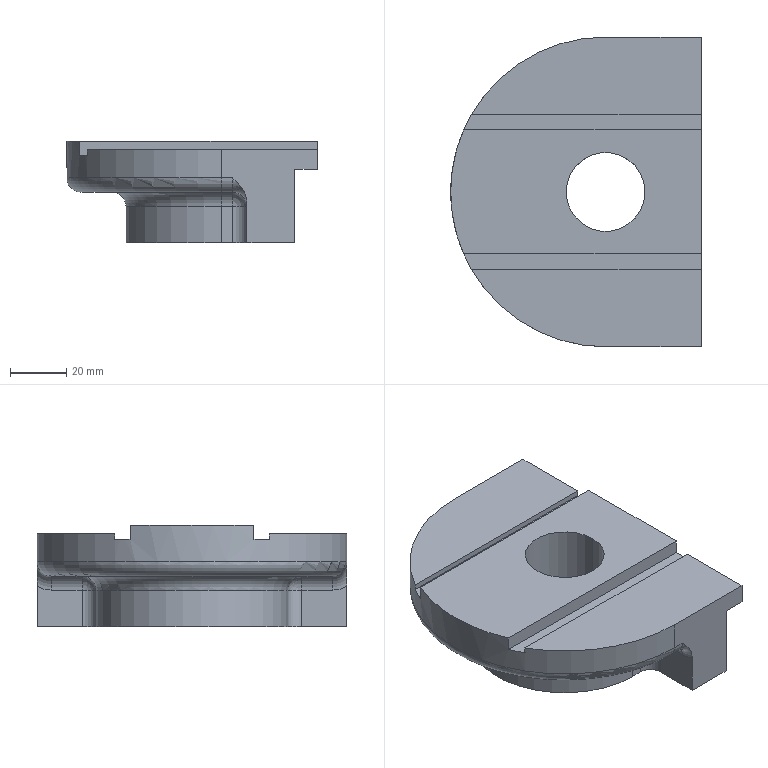Part | SolidWorks | features ICE 6, Fillet 3, Extrusion 1, MirrorPattern 1, RevCut 1 | 1 solid | 49 faces | box 89 x 110 x 36 mm | volume 178955 mm3 | plane 21 | cylinder 18 | cone 4 | torus 4 | sphere 2 | commonest cylinder face diameters 10 x8 5.5 x4 28 x2 36 x2 68 x1 110 x1
STEP:
#1=CARTESIAN_POINT('',(11.,-38.,-25.75));
#2=VERTEX_POINT('',#1);
#3=CARTESIAN_POINT('',(11.,-38.,-20.25));
#4=VERTEX_POINT('',#3);
#5=CARTESIAN_POINT('',(11.,-38.,-23.));
#6=DIRECTION('',(-1.,0.,0.));
#7=DIRECTION('',(0.,0.,-1.));
#8=AXIS2_PLACEMENT_3D('',#5,#6,#7);
#9=CIRCLE('',#8,2.75);
#10=EDGE_CURVE('',#2,#4,#9,.T.);
#11=ORIENTED_EDGE('',*,*,#10,.T.);
#12=CARTESIAN_POINT('',(26.,-38.,-20.25));
#13=VERTEX_POINT('',#12);
#14=CARTESIAN_POINT('',(29.177,-38.,-20.25));
#15=DIRECTION('',(1.,0.,0.));
#16=VECTOR('',#15,1000.);
#17=LINE('',#14,#16);
#18=EDGE_CURVE('',#4,#13,#17,.T.);
#19=ORIENTED_EDGE('',*,*,#18,.T.);
#20=CARTESIAN_POINT('',(26.,-38.,-25.75));
#21=VERTEX_POINT('',#20);
#22=CARTESIAN_POINT('',(26.,-38.,-23.));
#23=DIRECTION('',(-1.,0.,0.));
#24=DIRECTION('',(0.,0.,-1.));
#25=AXIS2_PLACEMENT_3D('',#22,#23,#24);
#26=CIRCLE('',#25,2.75);
#27=EDGE_CURVE('',#21,#13,#26,.T.);
#28=ORIENTED_EDGE('',*,*,#27,.F.);
#29=CARTESIAN_POINT('',(29.177,-38.,-25.75));
#30=DIRECTION('',(1.,0.,0.));
#31=VECTOR('',#30,1000.);
#32=LINE('',#29,#31);
#33=EDGE_CURVE('',#2,#21,#32,.T.);
#34=ORIENTED_EDGE('',*,*,#33,.F.);
#35=EDGE_LOOP('',(#11,#19,#28,#34));
#36=FACE_OUTER_BOUND('',#35,.T.);
#37=CARTESIAN_POINT('',(29.177,-38.,-23.));
#38=DIRECTION('',(1.,0.,0.));
#39=DIRECTION('',(0.,0.,-1.));
#40=AXIS2_PLACEMENT_3D('',#37,#38,#39);
#41=CYLINDRICAL_SURFACE('',#40,2.75);
#42=ADVANCED_FACE('',(#36),#41,.F.);
#43=CARTESIAN_POINT('',(9.412,-38.,-23.));
#44=VERTEX_POINT('',#43);
#45=CARTESIAN_POINT('',(9.412,-38.,-23.));
#46=DIRECTION('',(0.5,0.,-0.866));
#47=VECTOR('',#46,1000.);
#48=LINE('',#45,#47);
#49=EDGE_CURVE('',#44,#2,#48,.T.);
#50=ORIENTED_EDGE('',*,*,#49,.F.);
#51=CARTESIAN_POINT('',(9.412,-38.,-23.));
#52=DIRECTION('',(0.5,0.,0.866));
#53=VECTOR('',#52,1000.);
#54=LINE('',#51,#53);
#55=EDGE_CURVE('',#44,#4,#54,.T.);
#56=ORIENTED_EDGE('',*,*,#55,.T.);
#57=ORIENTED_EDGE('',*,*,#10,.F.);
#58=EDGE_LOOP('',(#50,#56,#57));
#59=FACE_OUTER_BOUND('',#58,.T.);
#60=CARTESIAN_POINT('',(1009.412,-38.,-23.));
#61=DIRECTION('',(1.,0.,0.));
#62=DIRECTION('',(0.,0.,-1.));
#63=AXIS2_PLACEMENT_3D('',#60,#61,#62);
#64=CONICAL_SURFACE('',#63,1732.051,1.047);
#65=ADVANCED_FACE('',(#59),#64,.F.);
#66=CARTESIAN_POINT('',(11.,38.,-20.25));
#67=VERTEX_POINT('',#66);
#68=CARTESIAN_POINT('',(11.,38.,-25.75));
#69=VERTEX_POINT('',#68);
#70=CARTESIAN_POINT('',(11.,38.,-23.));
#71=DIRECTION('',(1.,0.,0.));
#72=DIRECTION('',(0.,0.,-1.));
#73=AXIS2_PLACEMENT_3D('',#70,#71,#72);
#74=CIRCLE('',#73,2.75);
#75=EDGE_CURVE('',#67,#69,#74,.T.);
#76=ORIENTED_EDGE('',*,*,#75,.F.);
#77=CARTESIAN_POINT('',(26.,38.,-20.25));
#78=VERTEX_POINT('',#77);
#79=CARTESIAN_POINT('',(29.177,38.,-20.25));
#80=DIRECTION('',(1.,0.,0.));
#81=VECTOR('',#80,1000.);
#82=LINE('',#79,#81);
#83=EDGE_CURVE('',#67,#78,#82,.T.);
#84=ORIENTED_EDGE('',*,*,#83,.T.);
#85=CARTESIAN_POINT('',(26.,38.,-25.75));
#86=VERTEX_POINT('',#85);
#87=CARTESIAN_POINT('',(26.,38.,-23.));
#88=DIRECTION('',(1.,0.,0.));
#89=DIRECTION('',(0.,0.,-1.));
#90=AXIS2_PLACEMENT_3D('',#87,#88,#89);
#91=CIRCLE('',#90,2.75);
#92=EDGE_CURVE('',#78,#86,#91,.T.);
#93=ORIENTED_EDGE('',*,*,#92,.T.);
#94=CARTESIAN_POINT('',(29.177,38.,-25.75));
#95=DIRECTION('',(1.,0.,0.));
#96=VECTOR('',#95,1000.);
#97=LINE('',#94,#96);
#98=EDGE_CURVE('',#69,#86,#97,.T.);
#99=ORIENTED_EDGE('',*,*,#98,.F.);
#100=EDGE_LOOP('',(#76,#84,#93,#99));
#101=FACE_OUTER_BOUND('',#100,.T.);
#102=CARTESIAN_POINT('',(29.177,38.,-23.));
#103=DIRECTION('',(1.,0.,0.));
#104=DIRECTION('',(0.,0.,-1.));
#105=AXIS2_PLACEMENT_3D('',#102,#103,#104);
#106=CYLINDRICAL_SURFACE('',#105,2.75);
#107=ADVANCED_FACE('',(#101),#106,.F.);
#108=CARTESIAN_POINT('',(9.412,38.,-23.));
#109=VERTEX_POINT('',#108);
#110=CARTESIAN_POINT('',(9.412,38.,-23.));
#111=DIRECTION('',(0.5,0.,-0.866));
#112=VECTOR('',#111,1000.);
#113=LINE('',#110,#112);
#114=EDGE_CURVE('',#109,#69,#113,.T.);
#115=ORIENTED_EDGE('',*,*,#114,.F.);
#116=CARTESIAN_POINT('',(9.412,38.,-23.));
#117=DIRECTION('',(0.5,0.,0.866));
#118=VECTOR('',#117,1000.);
#119=LINE('',#116,#118);
#120=EDGE_CURVE('',#109,#67,#119,.T.);
#121=ORIENTED_EDGE('',*,*,#120,.T.);
#122=ORIENTED_EDGE('',*,*,#75,.T.);
#123=EDGE_LOOP('',(#115,#121,#122));
#124=FACE_OUTER_BOUND('',#123,.T.);
#125=CARTESIAN_POINT('',(1009.412,38.,-23.));
#126=DIRECTION('',(1.,0.,0.));
#127=DIRECTION('',(0.,0.,-1.));
#128=AXIS2_PLACEMENT_3D('',#125,#126,#127);
#129=CONICAL_SURFACE('',#128,1732.051,1.047);
#130=ADVANCED_FACE('',(#124),#129,.F.);
#131=CARTESIAN_POINT('',(18.,0.,-22.));
#132=VERTEX_POINT('',#131);
#133=CARTESIAN_POINT('',(-18.,0.,-22.));
#134=VERTEX_POINT('',#133);
#135=CARTESIAN_POINT('',(0.,0.,-22.));
#136=DIRECTION('',(0.,0.,-1.));
#137=DIRECTION('',(-1.,0.,0.));
#138=AXIS2_PLACEMENT_3D('',#135,#136,#137);
#139=CIRCLE('',#138,18.);
#140=EDGE_CURVE('',#132,#134,#139,.T.);
#141=ORIENTED_EDGE('',*,*,#140,.F.);
#142=CARTESIAN_POINT('',(18.,0.,-36.));
#143=VERTEX_POINT('',#142);
#144=CARTESIAN_POINT('',(18.,0.,-22.));
#145=DIRECTION('',(0.,0.,-1.));
#146=VECTOR('',#145,1000.);
#147=LINE('',#144,#146);
#148=EDGE_CURVE('',#132,#143,#147,.T.);
#149=ORIENTED_EDGE('',*,*,#148,.T.);
#150=CARTESIAN_POINT('',(-18.,0.,-36.));
#151=VERTEX_POINT('',#150);
#152=CARTESIAN_POINT('',(0.,0.,-36.));
#153=DIRECTION('',(0.,0.,-1.));
#154=DIRECTION('',(-1.,0.,0.));
#155=AXIS2_PLACEMENT_3D('',#152,#153,#154);
#156=CIRCLE('',#155,18.);
#157=EDGE_CURVE('',#143,#151,#156,.T.);
#158=ORIENTED_EDGE('',*,*,#157,.T.);
#159=CARTESIAN_POINT('',(-18.,0.,-22.));
#160=DIRECTION('',(0.,0.,-1.));
#161=VECTOR('',#160,1000.);
#162=LINE('',#159,#161);
#163=EDGE_CURVE('',#134,#151,#162,.T.);
#164=ORIENTED_EDGE('',*,*,#163,.F.);
#165=EDGE_LOOP('',(#141,#149,#158,#164));
#166=FACE_OUTER_BOUND('',#165,.T.);
#167=CARTESIAN_POINT('',(0.,0.,-22.));
#168=DIRECTION('',(0.,0.,-1.));
#169=DIRECTION('',(-1.,0.,0.));
#170=AXIS2_PLACEMENT_3D('',#167,#168,#169);
#171=CYLINDRICAL_SURFACE('',#170,18.);
#172=ADVANCED_FACE('',(#166),#171,.F.);
#173=CARTESIAN_POINT('',(-14.,0.,0.));
#174=VERTEX_POINT('',#173);
#175=CARTESIAN_POINT('',(14.,0.,0.));
#176=VERTEX_POINT('',#175);
#177=CARTESIAN_POINT('',(0.,0.,0.));
#178=DIRECTION('',(0.,0.,1.));
#179=DIRECTION('',(1.,0.,0.));
#180=AXIS2_PLACEMENT_3D('',#177,#178,#179);
#181=CIRCLE('',#180,14.);
#182=EDGE_CURVE('',#174,#176,#181,.T.);
#183=ORIENTED_EDGE('',*,*,#182,.T.);
#184=CARTESIAN_POINT('',(14.,0.,-22.));
#185=VERTEX_POINT('',#184);
#186=CARTESIAN_POINT('',(14.,0.,1.));
#187=DIRECTION('',(0.,0.,-1.));
#188=VECTOR('',#187,1000.);
#189=LINE('',#186,#188);
#190=EDGE_CURVE('',#176,#185,#189,.T.);
#191=ORIENTED_EDGE('',*,*,#190,.T.);
#192=CARTESIAN_POINT('',(-14.,0.,-22.));
#193=VERTEX_POINT('',#192);
#194=CARTESIAN_POINT('',(0.,0.,-22.));
#195=DIRECTION('',(0.,0.,1.));
#196=DIRECTION('',(-1.,0.,0.));
#197=AXIS2_PLACEMENT_3D('',#194,#195,#196);
#198=CIRCLE('',#197,14.);
#199=EDGE_CURVE('',#193,#185,#198,.T.);
#200=ORIENTED_EDGE('',*,*,#199,.F.);
#201=CARTESIAN_POINT('',(-14.,0.,1.));
#202=DIRECTION('',(0.,0.,-1.));
#203=VECTOR('',#202,1000.);
#204=LINE('',#201,#203);
#205=EDGE_CURVE('',#174,#193,#204,.T.);
#206=ORIENTED_EDGE('',*,*,#205,.F.);
#207=EDGE_LOOP('',(#183,#191,#200,#206));
#208=FACE_OUTER_BOUND('',#207,.T.);
#209=CARTESIAN_POINT('',(0.,0.,1.));
#210=DIRECTION('',(0.,0.,-1.));
#211=DIRECTION('',(-1.,0.,0.));
#212=AXIS2_PLACEMENT_3D('',#209,#210,#211);
#213=CYLINDRICAL_SURFACE('',#212,14.);
#214=ADVANCED_FACE('',(#208),#213,.F.);
#215=CARTESIAN_POINT('',(34.,-55.,-10.));
#216=VERTEX_POINT('',#215);
#217=CARTESIAN_POINT('',(34.,-55.,-3.));
#218=VERTEX_POINT('',#217);
#219=CARTESIAN_POINT('',(34.,-55.,-18.));
#220=DIRECTION('',(0.,0.,1.));
#221=VECTOR('',#220,1000.);
#222=LINE('',#219,#221);
#223=EDGE_CURVE('',#216,#218,#222,.T.);
#224=ORIENTED_EDGE('',*,*,#223,.F.);
#225=CARTESIAN_POINT('',(34.,55.,-10.));
#226=VERTEX_POINT('',#225);
#227=CARTESIAN_POINT('',(34.,55.,-10.));
#228=DIRECTION('',(0.,-1.,0.));
#229=VECTOR('',#228,1000.);
#230=LINE('',#227,#229);
#231=EDGE_CURVE('',#226,#216,#230,.T.);
#232=ORIENTED_EDGE('',*,*,#231,.F.);
#233=CARTESIAN_POINT('',(34.,55.,-3.));
#234=VERTEX_POINT('',#233);
#235=CARTESIAN_POINT('',(34.,55.,-18.));
#236=DIRECTION('',(0.,0.,1.));
#237=VECTOR('',#236,1000.);
#238=LINE('',#235,#237);
#239=EDGE_CURVE('',#226,#234,#238,.T.);
#240=ORIENTED_EDGE('',*,*,#239,.T.);
#241=CARTESIAN_POINT('',(34.,27.5,-3.));
#242=VERTEX_POINT('',#241);
#243=CARTESIAN_POINT('',(34.,55.,-3.));
#244=DIRECTION('',(0.,1.,0.));
#245=VECTOR('',#244,1000.);
#246=LINE('',#243,#245);
#247=EDGE_CURVE('',#242,#234,#246,.T.);
#248=ORIENTED_EDGE('',*,*,#247,.F.);
#249=CARTESIAN_POINT('',(34.,27.5,-5.));
#250=VERTEX_POINT('',#249);
#251=CARTESIAN_POINT('',(34.,27.5,0.));
#252=DIRECTION('',(0.,0.,1.));
#253=VECTOR('',#252,1000.);
#254=LINE('',#251,#253);
#255=EDGE_CURVE('',#250,#242,#254,.T.);
#256=ORIENTED_EDGE('',*,*,#255,.F.);
#257=CARTESIAN_POINT('',(34.,22.,-5.));
#258=VERTEX_POINT('',#257);
#259=CARTESIAN_POINT('',(34.,22.,-5.));
#260=DIRECTION('',(0.,1.,0.));
#261=VECTOR('',#260,1000.);
#262=LINE('',#259,#261);
#263=EDGE_CURVE('',#258,#250,#262,.T.);
#264=ORIENTED_EDGE('',*,*,#263,.F.);
#265=CARTESIAN_POINT('',(34.,22.,0.));
#266=VERTEX_POINT('',#265);
#267=CARTESIAN_POINT('',(34.,22.,0.));
#268=DIRECTION('',(0.,0.,-1.));
#269=VECTOR('',#268,1000.);
#270=LINE('',#267,#269);
#271=EDGE_CURVE('',#266,#258,#270,.T.);
#272=ORIENTED_EDGE('',*,*,#271,.F.);
#273=CARTESIAN_POINT('',(34.,-22.,0.));
#274=VERTEX_POINT('',#273);
#275=CARTESIAN_POINT('',(34.,55.,0.));
#276=DIRECTION('',(0.,1.,0.));
#277=VECTOR('',#276,1000.);
#278=LINE('',#275,#277);
#279=EDGE_CURVE('',#274,#266,#278,.T.);
#280=ORIENTED_EDGE('',*,*,#279,.F.);
#281=CARTESIAN_POINT('',(34.,-22.,-5.));
#282=VERTEX_POINT('',#281);
#283=CARTESIAN_POINT('',(34.,-22.,0.));
#284=DIRECTION('',(0.,0.,1.));
#285=VECTOR('',#284,1000.);
#286=LINE('',#283,#285);
#287=EDGE_CURVE('',#282,#274,#286,.T.);
#288=ORIENTED_EDGE('',*,*,#287,.F.);
#289=CARTESIAN_POINT('',(34.,-27.5,-5.));
#290=VERTEX_POINT('',#289);
#291=CARTESIAN_POINT('',(34.,-22.,-5.));
#292=DIRECTION('',(0.,1.,0.));
#293=VECTOR('',#292,1000.);
#294=LINE('',#291,#293);
#295=EDGE_CURVE('',#290,#282,#294,.T.);
#296=ORIENTED_EDGE('',*,*,#295,.F.);
#297=CARTESIAN_POINT('',(34.,-27.5,-3.));
#298=VERTEX_POINT('',#297);
#299=CARTESIAN_POINT('',(34.,-27.5,0.));
#300=DIRECTION('',(0.,0.,-1.));
#301=VECTOR('',#300,1000.);
#302=LINE('',#299,#301);
#303=EDGE_CURVE('',#298,#290,#302,.T.);
#304=ORIENTED_EDGE('',*,*,#303,.F.);
#305=CARTESIAN_POINT('',(34.,-55.,-3.));
#306=DIRECTION('',(0.,1.,0.));
#307=VECTOR('',#306,1000.);
#308=LINE('',#305,#307);
#309=EDGE_CURVE('',#218,#298,#308,.T.);
#310=ORIENTED_EDGE('',*,*,#309,.F.);
#311=EDGE_LOOP('',(#224,#232,#240,#248,#256,#264,#272,#280,#288,#296,#304,#310));
#312=FACE_OUTER_BOUND('',#311,.T.);
#313=CARTESIAN_POINT('',(34.,55.,-18.));
#314=DIRECTION('',(1.,0.,0.));
#315=DIRECTION('',(0.,1.,0.));
#316=AXIS2_PLACEMENT_3D('',#313,#314,#315);
#317=PLANE('',#316);
#318=ADVANCED_FACE('',(#312),#317,.T.);
#319=ORIENTED_EDGE('',*,*,#190,.F.);
#320=CARTESIAN_POINT('',(0.,0.,0.));
#321=DIRECTION('',(0.,0.,1.));
#322=DIRECTION('',(1.,0.,0.));
#323=AXIS2_PLACEMENT_3D('',#320,#321,#322);
#324=CIRCLE('',#323,14.);
#325=EDGE_CURVE('',#176,#174,#324,.T.);
#326=ORIENTED_EDGE('',*,*,#325,.T.);
#327=ORIENTED_EDGE('',*,*,#205,.T.);
#328=CARTESIAN_POINT('',(0.,0.,-22.));
#329=DIRECTION('',(0.,0.,1.));
#330=DIRECTION('',(-1.,0.,0.));
#331=AXIS2_PLACEMENT_3D('',#328,#329,#330);
#332=CIRCLE('',#331,14.);
#333=EDGE_CURVE('',#185,#193,#332,.T.);
#334=ORIENTED_EDGE('',*,*,#333,.F.);
#335=EDGE_LOOP('',(#319,#326,#327,#334));
#336=FACE_OUTER_BOUND('',#335,.T.);
#337=CARTESIAN_POINT('',(0.,0.,1.));
#338=DIRECTION('',(0.,0.,-1.));
#339=DIRECTION('',(-1.,0.,0.));
#340=AXIS2_PLACEMENT_3D('',#337,#338,#339);
#341=CYLINDRICAL_SURFACE('',#340,14.);
#342=ADVANCED_FACE('',(#336),#341,.F.);
#343=CARTESIAN_POINT('',(0.,-39.,-18.));
#344=VERTEX_POINT('',#343);
#345=CARTESIAN_POINT('',(4.,-39.,-18.));
#346=VERTEX_POINT('',#345);
#347=CARTESIAN_POINT('',(9.,-39.,-18.));
#348=DIRECTION('',(1.,0.,0.));
#349=VECTOR('',#348,1000.);
#350=LINE('',#347,#349);
#351=EDGE_CURVE('',#344,#346,#350,.T.);
#352=ORIENTED_EDGE('',*,*,#351,.T.);
#353=CARTESIAN_POINT('',(4.,-50.,-18.));
#354=VERTEX_POINT('',#353);
#355=CARTESIAN_POINT('',(4.,-50.,-18.));
#356=DIRECTION('',(0.,-1.,0.));
#357=VECTOR('',#356,1000.);
#358=LINE('',#355,#357);
#359=EDGE_CURVE('',#346,#354,#358,.T.);
#360=ORIENTED_EDGE('',*,*,#359,.T.);
#361=CARTESIAN_POINT('',(0.,-50.,-18.));
#362=VERTEX_POINT('',#361);
#363=CARTESIAN_POINT('',(0.,-50.,-18.));
#364=DIRECTION('',(-1.,0.,0.));
#365=VECTOR('',#364,1000.);
#366=LINE('',#363,#365);
#367=EDGE_CURVE('',#354,#362,#366,.T.);
#368=ORIENTED_EDGE('',*,*,#367,.T.);
#369=CARTESIAN_POINT('',(0.,50.,-18.));
#370=VERTEX_POINT('',#369);
#371=CARTESIAN_POINT('',(0.,0.,-18.));
#372=DIRECTION('',(0.,0.,-1.));
#373=DIRECTION('',(1.,0.,0.));
#374=AXIS2_PLACEMENT_3D('',#371,#372,#373);
#375=CIRCLE('',#374,50.);
#376=EDGE_CURVE('',#362,#370,#375,.T.);
#377=ORIENTED_EDGE('',*,*,#376,.T.);
#378=CARTESIAN_POINT('',(4.,50.,-18.));
#379=VERTEX_POINT('',#378);
#380=CARTESIAN_POINT('',(9.,50.,-18.));
#381=DIRECTION('',(1.,0.,0.));
#382=VECTOR('',#381,1000.);
#383=LINE('',#380,#382);
#384=EDGE_CURVE('',#370,#379,#383,.T.);
#385=ORIENTED_EDGE('',*,*,#384,.T.);
#386=CARTESIAN_POINT('',(4.,39.,-18.));
#387=VERTEX_POINT('',#386);
#388=CARTESIAN_POINT('',(4.,34.,-18.));
#389=DIRECTION('',(0.,-1.,0.));
#390=VECTOR('',#389,1000.);
#391=LINE('',#388,#390);
#392=EDGE_CURVE('',#379,#387,#391,.T.);
#393=ORIENTED_EDGE('',*,*,#392,.T.);
#394=CARTESIAN_POINT('',(0.,39.,-18.));
#395=VERTEX_POINT('',#394);
#396=CARTESIAN_POINT('',(0.,39.,-18.));
#397=DIRECTION('',(-1.,0.,0.));
#398=VECTOR('',#397,1000.);
#399=LINE('',#396,#398);
#400=EDGE_CURVE('',#387,#395,#399,.T.);
#401=ORIENTED_EDGE('',*,*,#400,.T.);
#402=CARTESIAN_POINT('',(0.,0.,-18.));
#403=DIRECTION('',(0.,0.,1.));
#404=DIRECTION('',(1.,0.,0.));
#405=AXIS2_PLACEMENT_3D('',#402,#403,#404);
#406=CIRCLE('',#405,39.);
#407=EDGE_CURVE('',#395,#344,#406,.T.);
#408=ORIENTED_EDGE('',*,*,#407,.T.);
#409=EDGE_LOOP('',(#352,#360,#368,#377,#385,#393,#401,#408));
#410=FACE_OUTER_BOUND('',#409,.T.);
#411=CARTESIAN_POINT('',(0.,0.,-18.));
#412=DIRECTION('',(0.,0.,1.));
#413=DIRECTION('',(1.,0.,0.));
#414=AXIS2_PLACEMENT_3D('',#411,#412,#413);
#415=PLANE('',#414);
#416=ADVANCED_FACE('',(#410),#415,.F.);
#417=CARTESIAN_POINT('',(-47.631,27.5,-3.));
#418=VERTEX_POINT('',#417);
#419=CARTESIAN_POINT('',(-47.631,27.5,-5.));
#420=VERTEX_POINT('',#419);
#421=CARTESIAN_POINT('',(-47.631,27.5,-18.));
#422=DIRECTION('',(0.,0.,-1.));
#423=VECTOR('',#422,1000.);
#424=LINE('',#421,#423);
#425=EDGE_CURVE('',#418,#420,#424,.T.);
#426=ORIENTED_EDGE('',*,*,#425,.F.);
#427=CARTESIAN_POINT('',(0.,55.,-3.));
#428=VERTEX_POINT('',#427);
#429=CARTESIAN_POINT('',(0.,0.,-3.));
#430=DIRECTION('',(0.,0.,1.));
#431=DIRECTION('',(0.,1.,0.));
#432=AXIS2_PLACEMENT_3D('',#429,#430,#431);
#433=CIRCLE('',#432,55.);
#434=EDGE_CURVE('',#428,#418,#433,.T.);
#435=ORIENTED_EDGE('',*,*,#434,.F.);
#436=CARTESIAN_POINT('',(0.,55.,-13.));
#437=VERTEX_POINT('',#436);
#438=CARTESIAN_POINT('',(0.,55.,-18.));
#439=DIRECTION('',(0.,0.,1.));
#440=VECTOR('',#439,1000.);
#441=LINE('',#438,#440);
#442=EDGE_CURVE('',#437,#428,#441,.T.);
#443=ORIENTED_EDGE('',*,*,#442,.F.);
#444=CARTESIAN_POINT('',(0.,-55.,-13.));
#445=VERTEX_POINT('',#444);
#446=CARTESIAN_POINT('',(0.,0.,-13.));
#447=DIRECTION('',(0.,0.,1.));
#448=DIRECTION('',(1.,0.,0.));
#449=AXIS2_PLACEMENT_3D('',#446,#447,#448);
#450=CIRCLE('',#449,55.);
#451=EDGE_CURVE('',#437,#445,#450,.T.);
#452=ORIENTED_EDGE('',*,*,#451,.T.);
#453=CARTESIAN_POINT('',(0.,-55.,-3.));
#454=VERTEX_POINT('',#453);
#455=CARTESIAN_POINT('',(0.,-55.,-18.));
#456=DIRECTION('',(0.,0.,1.));
#457=VECTOR('',#456,1000.);
#458=LINE('',#455,#457);
#459=EDGE_CURVE('',#445,#454,#458,.T.);
#460=ORIENTED_EDGE('',*,*,#459,.T.);
#461=CARTESIAN_POINT('',(-47.631,-27.5,-3.));
#462=VERTEX_POINT('',#461);
#463=CARTESIAN_POINT('',(0.,0.,-3.));
#464=DIRECTION('',(0.,0.,1.));
#465=DIRECTION('',(0.,1.,0.));
#466=AXIS2_PLACEMENT_3D('',#463,#464,#465);
#467=CIRCLE('',#466,55.);
#468=EDGE_CURVE('',#462,#454,#467,.T.);
#469=ORIENTED_EDGE('',*,*,#468,.F.);
#470=CARTESIAN_POINT('',(-47.631,-27.5,-5.));
#471=VERTEX_POINT('',#470);
#472=CARTESIAN_POINT('',(-47.631,-27.5,-18.));
#473=DIRECTION('',(0.,0.,1.));
#474=VECTOR('',#473,1000.);
#475=LINE('',#472,#474);
#476=EDGE_CURVE('',#471,#462,#475,.T.);
#477=ORIENTED_EDGE('',*,*,#476,.F.);
#478=CARTESIAN_POINT('',(-50.408,-22.,-5.));
#479=VERTEX_POINT('',#478);
#480=CARTESIAN_POINT('',(0.,0.,-5.));
#481=DIRECTION('',(0.,0.,1.));
#482=DIRECTION('',(-1.,0.,0.));
#483=AXIS2_PLACEMENT_3D('',#480,#481,#482);
#484=CIRCLE('',#483,55.);
#485=EDGE_CURVE('',#479,#471,#484,.T.);
#486=ORIENTED_EDGE('',*,*,#485,.F.);
#487=CARTESIAN_POINT('',(-50.408,-22.,0.));
#488=VERTEX_POINT('',#487);
#489=CARTESIAN_POINT('',(-50.408,-22.,-18.));
#490=DIRECTION('',(0.,0.,-1.));
#491=VECTOR('',#490,1000.);
#492=LINE('',#489,#491);
#493=EDGE_CURVE('',#488,#479,#492,.T.);
#494=ORIENTED_EDGE('',*,*,#493,.F.);
#495=CARTESIAN_POINT('',(-50.408,22.,0.));
#496=VERTEX_POINT('',#495);
#497=CARTESIAN_POINT('',(0.,0.,0.));
#498=DIRECTION('',(0.,0.,1.));
#499=DIRECTION('',(1.,0.,0.));
#500=AXIS2_PLACEMENT_3D('',#497,#498,#499);
#501=CIRCLE('',#500,55.);
#502=EDGE_CURVE('',#496,#488,#501,.T.);
#503=ORIENTED_EDGE('',*,*,#502,.F.);
#504=CARTESIAN_POINT('',(-50.408,22.,-5.));
#505=VERTEX_POINT('',#504);
#506=CARTESIAN_POINT('',(-50.408,22.,-18.));
#507=DIRECTION('',(0.,0.,1.));
#508=VECTOR('',#507,1000.);
#509=LINE('',#506,#508);
#510=EDGE_CURVE('',#505,#496,#509,.T.);
#511=ORIENTED_EDGE('',*,*,#510,.F.);
#512=CARTESIAN_POINT('',(0.,0.,-5.));
#513=DIRECTION('',(0.,0.,1.));
#514=DIRECTION('',(-1.,0.,0.));
#515=AXIS2_PLACEMENT_3D('',#512,#513,#514);
#516=CIRCLE('',#515,55.);
#517=EDGE_CURVE('',#420,#505,#516,.T.);
#518=ORIENTED_EDGE('',*,*,#517,.F.);
#519=EDGE_LOOP('',(#426,#435,#443,#452,#460,#469,#477,#486,#494,#503,#511,#518));
#520=FACE_OUTER_BOUND('',#519,.T.);
#521=CARTESIAN_POINT('',(0.,0.,-18.));
#522=DIRECTION('',(0.,0.,1.));
#523=DIRECTION('',(1.,0.,0.));
#524=AXIS2_PLACEMENT_3D('',#521,#522,#523);
#525=CYLINDRICAL_SURFACE('',#524,55.);
#526=ADVANCED_FACE('',(#520),#525,.T.);
#527=CARTESIAN_POINT('',(26.,55.,-10.));
#528=VERTEX_POINT('',#527);
#529=CARTESIAN_POINT('',(34.,55.,-10.));
#530=DIRECTION('',(1.,0.,0.));
#531=VECTOR('',#530,1000.);
#532=LINE('',#529,#531);
#533=EDGE_CURVE('',#528,#226,#532,.T.);
#534=ORIENTED_EDGE('',*,*,#533,.F.);
#535=CARTESIAN_POINT('',(26.,55.,-36.));
#536=VERTEX_POINT('',#535);
#537=CARTESIAN_POINT('',(26.,55.,-36.));
#538=DIRECTION('',(0.,0.,1.));
#539=VECTOR('',#538,1000.);
#540=LINE('',#537,#539);
#541=EDGE_CURVE('',#536,#528,#540,.T.);
#542=ORIENTED_EDGE('',*,*,#541,.F.);
#543=CARTESIAN_POINT('',(9.,55.,-36.));
#544=VERTEX_POINT('',#543);
#545=CARTESIAN_POINT('',(9.,55.,-36.));
#546=DIRECTION('',(1.,0.,0.));
#547=VECTOR('',#546,1000.);
#548=LINE('',#545,#547);
#549=EDGE_CURVE('',#544,#536,#548,.T.);
#550=ORIENTED_EDGE('',*,*,#549,.F.);
#551=CARTESIAN_POINT('',(9.,55.,-21.66));
#552=VERTEX_POINT('',#551);
#553=CARTESIAN_POINT('',(9.,55.,-36.));
#554=DIRECTION('',(0.,0.,1.));
#555=VECTOR('',#554,1000.);
#556=LINE('',#553,#555);
#557=EDGE_CURVE('',#544,#552,#556,.T.);
#558=ORIENTED_EDGE('',*,*,#557,.T.);
#559=CARTESIAN_POINT('',(4.,55.,-13.));
#560=VERTEX_POINT('',#559);
#561=CARTESIAN_POINT('',(9.,55.,-21.66));
#562=CARTESIAN_POINT('',(9.,55.,-20.794));
#563=CARTESIAN_POINT('',(8.836,55.,-19.956));
#564=CARTESIAN_POINT('',(8.258,55.,-18.327));
#565=CARTESIAN_POINT('',(7.857,55.,-17.575));
#566=CARTESIAN_POINT('',(7.147,55.,-16.508));
#567=CARTESIAN_POINT('',(6.891,55.,-16.162));
#568=CARTESIAN_POINT('',(6.355,55.,-15.491));
#569=CARTESIAN_POINT('',(6.076,55.,-15.166));
#570=CARTESIAN_POINT('',(5.501,55.,-14.531));
#571=CARTESIAN_POINT('',(5.205,55.,-14.22));
#572=CARTESIAN_POINT('',(4.606,55.,-13.606));
#573=CARTESIAN_POINT('',(4.302,55.,-13.302));
#574=CARTESIAN_POINT('',(4.,55.,-13.));
#575=B_SPLINE_CURVE_WITH_KNOTS('',3,(#561,#562,#563,#564,#565,#566,#567,#568,#569,#570,#571,#572,#573,#574),.UNSPECIFIED.,.F.,.F.,(4,2,2,2,2,2,4),(0.,0.002559,0.005119,0.006398,0.007678,0.008958,0.01024),.UNSPECIFIED.);
#576=EDGE_CURVE('',#552,#560,#575,.T.);
#577=ORIENTED_EDGE('',*,*,#576,.T.);
#578=CARTESIAN_POINT('',(0.,55.,-13.));
#579=DIRECTION('',(-1.,0.,0.));
#580=VECTOR('',#579,1000.);
#581=LINE('',#578,#580);
#582=EDGE_CURVE('',#560,#437,#581,.T.);
#583=ORIENTED_EDGE('',*,*,#582,.T.);
#584=ORIENTED_EDGE('',*,*,#442,.T.);
#585=CARTESIAN_POINT('',(-70.,55.,-3.));
#586=DIRECTION('',(1.,0.,0.));
#587=VECTOR('',#586,1000.);
#588=LINE('',#585,#587);
#589=EDGE_CURVE('',#428,#234,#588,.T.);
#590=ORIENTED_EDGE('',*,*,#589,.T.);
#591=ORIENTED_EDGE('',*,*,#239,.F.);
#592=EDGE_LOOP('',(#534,#542,#550,#558,#577,#583,#584,#590,#591));
#593=FACE_OUTER_BOUND('',#592,.T.);
#594=CARTESIAN_POINT('',(0.,55.,-18.));
#595=DIRECTION('',(0.,1.,0.));
#596=DIRECTION('',(0.,0.,1.));
#597=AXIS2_PLACEMENT_3D('',#594,#595,#596);
#598=PLANE('',#597);
#599=ADVANCED_FACE('',(#593),#598,.T.);
#600=CARTESIAN_POINT('',(26.,-55.,-36.));
#601=VERTEX_POINT('',#600);
#602=CARTESIAN_POINT('',(26.,-55.,-10.));
#603=VERTEX_POINT('',#602);
#604=CARTESIAN_POINT('',(26.,-55.,-36.));
#605=DIRECTION('',(0.,0.,1.));
#606=VECTOR('',#605,1000.);
#607=LINE('',#604,#606);
#608=EDGE_CURVE('',#601,#603,#607,.T.);
#609=ORIENTED_EDGE('',*,*,#608,.T.);
#610=CARTESIAN_POINT('',(34.,-55.,-10.));
#611=DIRECTION('',(-1.,0.,0.));
#612=VECTOR('',#611,1000.);
#613=LINE('',#610,#612);
#614=EDGE_CURVE('',#216,#603,#613,.T.);
#615=ORIENTED_EDGE('',*,*,#614,.F.);
#616=ORIENTED_EDGE('',*,*,#223,.T.);
#617=CARTESIAN_POINT('',(-70.,-55.,-3.));
#618=DIRECTION('',(1.,0.,0.));
#619=VECTOR('',#618,1000.);
#620=LINE('',#617,#619);
#621=EDGE_CURVE('',#454,#218,#620,.T.);
#622=ORIENTED_EDGE('',*,*,#621,.F.);
#623=ORIENTED_EDGE('',*,*,#459,.F.);
#624=CARTESIAN_POINT('',(4.,-55.,-13.));
#625=VERTEX_POINT('',#624);
#626=CARTESIAN_POINT('',(9.,-55.,-13.));
#627=DIRECTION('',(1.,0.,0.));
#628=VECTOR('',#627,1000.);
#629=LINE('',#626,#628);
#630=EDGE_CURVE('',#445,#625,#629,.T.);
#631=ORIENTED_EDGE('',*,*,#630,.T.);
#632=CARTESIAN_POINT('',(9.,-55.,-21.66));
#633=VERTEX_POINT('',#632);
#634=CARTESIAN_POINT('',(4.,-55.,-13.));
#635=CARTESIAN_POINT('',(4.606,-55.,-13.606));
#636=CARTESIAN_POINT('',(5.213,-55.,-14.213));
#637=CARTESIAN_POINT('',(6.076,-55.,-15.166));
#638=CARTESIAN_POINT('',(6.355,-55.,-15.491));
#639=CARTESIAN_POINT('',(6.891,-55.,-16.162));
#640=CARTESIAN_POINT('',(7.147,-55.,-16.508));
#641=CARTESIAN_POINT('',(7.857,-55.,-17.575));
#642=CARTESIAN_POINT('',(8.258,-55.,-18.327));
#643=CARTESIAN_POINT('',(8.836,-55.,-19.956));
#644=CARTESIAN_POINT('',(9.,-55.,-20.794));
#645=CARTESIAN_POINT('',(9.,-55.,-21.66));
#646=B_SPLINE_CURVE_WITH_KNOTS('',3,(#634,#635,#636,#637,#638,#639,#640,#641,#642,#643,#644,#645),.UNSPECIFIED.,.F.,.F.,(4,2,2,2,2,4),(-0.00001414,0.002557,0.003842,0.005127,0.007698,0.01027),.UNSPECIFIED.);
#647=EDGE_CURVE('',#625,#633,#646,.T.);
#648=ORIENTED_EDGE('',*,*,#647,.T.);
#649=CARTESIAN_POINT('',(9.,-55.,-36.));
#650=VERTEX_POINT('',#649);
#651=CARTESIAN_POINT('',(9.,-55.,-36.));
#652=DIRECTION('',(0.,0.,1.));
#653=VECTOR('',#652,1000.);
#654=LINE('',#651,#653);
#655=EDGE_CURVE('',#650,#633,#654,.T.);
#656=ORIENTED_EDGE('',*,*,#655,.F.);
#657=CARTESIAN_POINT('',(9.,-55.,-36.));
#658=DIRECTION('',(-1.,0.,0.));
#659=VECTOR('',#658,1000.);
#660=LINE('',#657,#659);
#661=EDGE_CURVE('',#601,#650,#660,.T.);
#662=ORIENTED_EDGE('',*,*,#661,.F.);
#663=EDGE_LOOP('',(#609,#615,#616,#622,#623,#631,#648,#656,#662));
#664=FACE_OUTER_BOUND('',#663,.T.);
#665=CARTESIAN_POINT('',(0.,-55.,-18.));
#666=DIRECTION('',(0.,-1.,0.));
#667=DIRECTION('',(0.,0.,-1.));
#668=AXIS2_PLACEMENT_3D('',#665,#666,#667);
#669=PLANE('',#668);
#670=ADVANCED_FACE('',(#664),#669,.T.);
#671=CARTESIAN_POINT('',(0.,22.,0.));
#672=DIRECTION('',(1.,0.,0.));
#673=VECTOR('',#672,1000.);
#674=LINE('',#671,#673);
#675=EDGE_CURVE('',#496,#266,#674,.T.);
#676=ORIENTED_EDGE('',*,*,#675,.F.);
#677=ORIENTED_EDGE('',*,*,#502,.T.);
#678=CARTESIAN_POINT('',(0.,-22.,0.));
#679=DIRECTION('',(-1.,0.,0.));
#680=VECTOR('',#679,1000.);
#681=LINE('',#678,#680);
#682=EDGE_CURVE('',#274,#488,#681,.T.);
#683=ORIENTED_EDGE('',*,*,#682,.F.);
#684=ORIENTED_EDGE('',*,*,#279,.T.);
#685=EDGE_LOOP('',(#676,#677,#683,#684));
#686=FACE_OUTER_BOUND('',#685,.T.);
#687=ORIENTED_EDGE('',*,*,#182,.F.);
#688=ORIENTED_EDGE('',*,*,#325,.F.);
#689=EDGE_LOOP('',(#687,#688));
#690=FACE_BOUND('',#689,.T.);
#691=CARTESIAN_POINT('',(0.,0.,0.));
#692=DIRECTION('',(0.,0.,1.));
#693=DIRECTION('',(1.,0.,0.));
#694=AXIS2_PLACEMENT_3D('',#691,#692,#693);
#695=PLANE('',#694);
#696=ADVANCED_FACE('',(#686,#690),#695,.T.);
#697=CARTESIAN_POINT('',(0.,-34.,-36.));
#698=VERTEX_POINT('',#697);
#699=CARTESIAN_POINT('',(0.,-34.,-23.));
#700=VERTEX_POINT('',#699);
#701=CARTESIAN_POINT('',(0.,-34.,-36.));
#702=DIRECTION('',(0.,0.,1.));
#703=VECTOR('',#702,1000.);
#704=LINE('',#701,#703);
#705=EDGE_CURVE('',#698,#700,#704,.T.);
#706=ORIENTED_EDGE('',*,*,#705,.T.);
#707=CARTESIAN_POINT('',(0.,34.,-23.));
#708=VERTEX_POINT('',#707);
#709=CARTESIAN_POINT('',(0.,0.,-23.));
#710=DIRECTION('',(0.,0.,-1.));
#711=DIRECTION('',(1.,0.,0.));
#712=AXIS2_PLACEMENT_3D('',#709,#710,#711);
#713=CIRCLE('',#712,34.);
#714=EDGE_CURVE('',#700,#708,#713,.T.);
#715=ORIENTED_EDGE('',*,*,#714,.T.);
#716=CARTESIAN_POINT('',(0.,34.,-36.));
#717=VERTEX_POINT('',#716);
#718=CARTESIAN_POINT('',(0.,34.,-36.));
#719=DIRECTION('',(0.,0.,1.));
#720=VECTOR('',#719,1000.);
#721=LINE('',#718,#720);
#722=EDGE_CURVE('',#717,#708,#721,.T.);
#723=ORIENTED_EDGE('',*,*,#722,.F.);
#724=CARTESIAN_POINT('',(0.,0.,-36.));
#725=DIRECTION('',(0.,0.,-1.));
#726=DIRECTION('',(-1.,0.,0.));
#727=AXIS2_PLACEMENT_3D('',#724,#725,#726);
#728=CIRCLE('',#727,34.);
#729=EDGE_CURVE('',#698,#717,#728,.T.);
#730=ORIENTED_EDGE('',*,*,#729,.F.);
#731=EDGE_LOOP('',(#706,#715,#723,#730));
#732=FACE_OUTER_BOUND('',#731,.T.);
#733=CARTESIAN_POINT('',(0.,0.,-36.));
#734=DIRECTION('',(0.,0.,1.));
#735=DIRECTION('',(1.,0.,0.));
#736=AXIS2_PLACEMENT_3D('',#733,#734,#735);
#737=CYLINDRICAL_SURFACE('',#736,34.);
#738=ADVANCED_FACE('',(#732),#737,.T.);
#739=CARTESIAN_POINT('',(4.,34.,-23.));
#740=VERTEX_POINT('',#739);
#741=CARTESIAN_POINT('',(9.,34.,-23.));
#742=DIRECTION('',(1.,0.,0.));
#743=VECTOR('',#742,1000.);
#744=LINE('',#741,#743);
#745=EDGE_CURVE('',#708,#740,#744,.T.);
#746=ORIENTED_EDGE('',*,*,#745,.T.);
#747=CARTESIAN_POINT('',(4.,34.,-36.));
#748=VERTEX_POINT('',#747);
#749=CARTESIAN_POINT('',(4.,34.,-36.));
#750=DIRECTION('',(0.,0.,-1.));
#751=VECTOR('',#750,1000.);
#752=LINE('',#749,#751);
#753=EDGE_CURVE('',#740,#748,#752,.T.);
#754=ORIENTED_EDGE('',*,*,#753,.T.);
#755=CARTESIAN_POINT('',(0.,34.,-36.));
#756=DIRECTION('',(1.,0.,0.));
#757=VECTOR('',#756,1000.);
#758=LINE('',#755,#757);
#759=EDGE_CURVE('',#717,#748,#758,.T.);
#760=ORIENTED_EDGE('',*,*,#759,.F.);
#761=ORIENTED_EDGE('',*,*,#722,.T.);
#762=EDGE_LOOP('',(#746,#754,#760,#761));
#763=FACE_OUTER_BOUND('',#762,.T.);
#764=CARTESIAN_POINT('',(0.,34.,-36.));
#765=DIRECTION('',(0.,-1.,0.));
#766=DIRECTION('',(0.,0.,-1.));
#767=AXIS2_PLACEMENT_3D('',#764,#765,#766);
#768=PLANE('',#767);
#769=ADVANCED_FACE('',(#763),#768,.F.);
#770=CARTESIAN_POINT('',(9.,39.,-36.));
#771=VERTEX_POINT('',#770);
#772=CARTESIAN_POINT('',(9.,34.,-36.));
#773=DIRECTION('',(0.,1.,0.));
#774=VECTOR('',#773,1000.);
#775=LINE('',#772,#774);
#776=EDGE_CURVE('',#771,#544,#775,.T.);
#777=ORIENTED_EDGE('',*,*,#776,.F.);
#778=CARTESIAN_POINT('',(9.,39.,-23.));
#779=VERTEX_POINT('',#778);
#780=CARTESIAN_POINT('',(9.,39.,-23.));
#781=DIRECTION('',(0.,0.,1.));
#782=VECTOR('',#781,1000.);
#783=LINE('',#780,#782);
#784=EDGE_CURVE('',#771,#779,#783,.T.);
#785=ORIENTED_EDGE('',*,*,#784,.T.);
#786=CARTESIAN_POINT('',(9.,50.,-23.));
#787=VERTEX_POINT('',#786);
#788=CARTESIAN_POINT('',(9.,50.,-23.));
#789=DIRECTION('',(0.,1.,0.));
#790=VECTOR('',#789,1000.);
#791=LINE('',#788,#790);
#792=EDGE_CURVE('',#779,#787,#791,.T.);
#793=ORIENTED_EDGE('',*,*,#792,.T.);
#794=CARTESIAN_POINT('',(9.,50.,-13.));
#795=DIRECTION('',(1.,0.,0.));
#796=DIRECTION('',(0.,0.,-1.));
#797=AXIS2_PLACEMENT_3D('',#794,#795,#796);
#798=CIRCLE('',#797,10.);
#799=EDGE_CURVE('',#787,#552,#798,.T.);
#800=ORIENTED_EDGE('',*,*,#799,.T.);
#801=ORIENTED_EDGE('',*,*,#557,.F.);
#802=EDGE_LOOP('',(#777,#785,#793,#800,#801));
#803=FACE_OUTER_BOUND('',#802,.T.);
#804=CARTESIAN_POINT('',(9.,34.,-36.));
#805=DIRECTION('',(1.,0.,0.));
#806=DIRECTION('',(0.,0.,-1.));
#807=AXIS2_PLACEMENT_3D('',#804,#805,#806);
#808=PLANE('',#807);
#809=ADVANCED_FACE('',(#803),#808,.F.);
#810=ORIENTED_EDGE('',*,*,#27,.T.);
#811=CARTESIAN_POINT('',(26.,-38.,-23.));
#812=DIRECTION('',(-1.,0.,0.));
#813=DIRECTION('',(0.,0.,-1.));
#814=AXIS2_PLACEMENT_3D('',#811,#812,#813);
#815=CIRCLE('',#814,2.75);
#816=EDGE_CURVE('',#13,#21,#815,.T.);
#817=ORIENTED_EDGE('',*,*,#816,.T.);
#818=EDGE_LOOP('',(#810,#817));
#819=FACE_BOUND('',#818,.T.);
#820=CARTESIAN_POINT('',(26.,38.,-23.));
#821=DIRECTION('',(1.,0.,0.));
#822=DIRECTION('',(0.,0.,-1.));
#823=AXIS2_PLACEMENT_3D('',#820,#821,#822);
#824=CIRCLE('',#823,2.75);
#825=EDGE_CURVE('',#86,#78,#824,.T.);
#826=ORIENTED_EDGE('',*,*,#825,.F.);
#827=ORIENTED_EDGE('',*,*,#92,.F.);
#828=EDGE_LOOP('',(#826,#827));
#829=FACE_BOUND('',#828,.T.);
#830=ORIENTED_EDGE('',*,*,#541,.T.);
#831=CARTESIAN_POINT('',(26.,55.,-10.));
#832=DIRECTION('',(0.,1.,0.));
#833=VECTOR('',#832,1000.);
#834=LINE('',#831,#833);
#835=EDGE_CURVE('',#603,#528,#834,.T.);
#836=ORIENTED_EDGE('',*,*,#835,.F.);
#837=ORIENTED_EDGE('',*,*,#608,.F.);
#838=CARTESIAN_POINT('',(26.,55.,-36.));
#839=DIRECTION('',(0.,-1.,0.));
#840=VECTOR('',#839,1000.);
#841=LINE('',#838,#840);
#842=EDGE_CURVE('',#536,#601,#841,.T.);
#843=ORIENTED_EDGE('',*,*,#842,.F.);
#844=EDGE_LOOP('',(#830,#836,#837,#843));
#845=FACE_OUTER_BOUND('',#844,.T.);
#846=CARTESIAN_POINT('',(26.,55.,-36.));
#847=DIRECTION('',(-1.,0.,0.));
#848=DIRECTION('',(0.,-1.,0.));
#849=AXIS2_PLACEMENT_3D('',#846,#847,#848);
#850=PLANE('',#849);
#851=ADVANCED_FACE('',(#819,#829,#845),#850,.F.);
#852=CARTESIAN_POINT('',(9.,-50.,-23.));
#853=VERTEX_POINT('',#852);
#854=CARTESIAN_POINT('',(9.,-39.,-23.));
#855=VERTEX_POINT('',#854);
#856=CARTESIAN_POINT('',(9.,-34.,-23.));
#857=DIRECTION('',(0.,1.,0.));
#858=VECTOR('',#857,1000.);
#859=LINE('',#856,#858);
#860=EDGE_CURVE('',#853,#855,#859,.T.);
#861=ORIENTED_EDGE('',*,*,#860,.T.);
#862=CARTESIAN_POINT('',(9.,-39.,-36.));
#863=VERTEX_POINT('',#862);
#864=CARTESIAN_POINT('',(9.,-39.,-36.));
#865=DIRECTION('',(0.,0.,-1.));
#866=VECTOR('',#865,1000.);
#867=LINE('',#864,#866);
#868=EDGE_CURVE('',#855,#863,#867,.T.);
#869=ORIENTED_EDGE('',*,*,#868,.T.);
#870=CARTESIAN_POINT('',(9.,-34.,-36.));
#871=DIRECTION('',(0.,1.,0.));
#872=VECTOR('',#871,1000.);
#873=LINE('',#870,#872);
#874=EDGE_CURVE('',#650,#863,#873,.T.);
#875=ORIENTED_EDGE('',*,*,#874,.F.);
#876=ORIENTED_EDGE('',*,*,#655,.T.);
#877=CARTESIAN_POINT('',(9.,-50.,-13.));
#878=DIRECTION('',(1.,0.,0.));
#879=DIRECTION('',(0.,1.,0.));
#880=AXIS2_PLACEMENT_3D('',#877,#878,#879);
#881=CIRCLE('',#880,10.);
#882=EDGE_CURVE('',#633,#853,#881,.T.);
#883=ORIENTED_EDGE('',*,*,#882,.T.);
#884=EDGE_LOOP('',(#861,#869,#875,#876,#883));
#885=FACE_OUTER_BOUND('',#884,.T.);
#886=CARTESIAN_POINT('',(9.,-34.,-36.));
#887=DIRECTION('',(1.,0.,0.));
#888=DIRECTION('',(0.,1.,0.));
#889=AXIS2_PLACEMENT_3D('',#886,#887,#888);
#890=PLANE('',#889);
#891=ADVANCED_FACE('',(#885),#890,.F.);
#892=CARTESIAN_POINT('',(4.,-34.,-36.));
#893=VERTEX_POINT('',#892);
#894=CARTESIAN_POINT('',(0.,-34.,-36.));
#895=DIRECTION('',(-1.,0.,0.));
#896=VECTOR('',#895,1000.);
#897=LINE('',#894,#896);
#898=EDGE_CURVE('',#893,#698,#897,.T.);
#899=ORIENTED_EDGE('',*,*,#898,.F.);
#900=CARTESIAN_POINT('',(4.,-34.,-23.));
#901=VERTEX_POINT('',#900);
#902=CARTESIAN_POINT('',(4.,-34.,-23.));
#903=DIRECTION('',(0.,0.,1.));
#904=VECTOR('',#903,1000.);
#905=LINE('',#902,#904);
#906=EDGE_CURVE('',#893,#901,#905,.T.);
#907=ORIENTED_EDGE('',*,*,#906,.T.);
#908=CARTESIAN_POINT('',(0.,-34.,-23.));
#909=DIRECTION('',(-1.,0.,0.));
#910=VECTOR('',#909,1000.);
#911=LINE('',#908,#910);
#912=EDGE_CURVE('',#901,#700,#911,.T.);
#913=ORIENTED_EDGE('',*,*,#912,.T.);
#914=ORIENTED_EDGE('',*,*,#705,.F.);
#915=EDGE_LOOP('',(#899,#907,#913,#914));
#916=FACE_OUTER_BOUND('',#915,.T.);
#917=CARTESIAN_POINT('',(0.,-34.,-36.));
#918=DIRECTION('',(0.,1.,0.));
#919=DIRECTION('',(0.,0.,1.));
#920=AXIS2_PLACEMENT_3D('',#917,#918,#919);
#921=PLANE('',#920);
#922=ADVANCED_FACE('',(#916),#921,.F.);
#923=CARTESIAN_POINT('',(0.,0.,-36.));
#924=DIRECTION('',(0.,0.,-1.));
#925=DIRECTION('',(-1.,0.,0.));
#926=AXIS2_PLACEMENT_3D('',#923,#924,#925);
#927=CIRCLE('',#926,18.);
#928=EDGE_CURVE('',#151,#143,#927,.T.);
#929=ORIENTED_EDGE('',*,*,#928,.F.);
#930=ORIENTED_EDGE('',*,*,#157,.F.);
#931=EDGE_LOOP('',(#929,#930));
#932=FACE_BOUND('',#931,.T.);
#933=ORIENTED_EDGE('',*,*,#729,.T.);
#934=ORIENTED_EDGE('',*,*,#759,.T.);
#935=CARTESIAN_POINT('',(4.,39.,-36.));
#936=DIRECTION('',(0.,0.,1.));
#937=DIRECTION('',(-1.,0.,0.));
#938=AXIS2_PLACEMENT_3D('',#935,#936,#937);
#939=CIRCLE('',#938,5.);
#940=EDGE_CURVE('',#748,#771,#939,.T.);
#941=ORIENTED_EDGE('',*,*,#940,.T.);
#942=ORIENTED_EDGE('',*,*,#776,.T.);
#943=ORIENTED_EDGE('',*,*,#549,.T.);
#944=ORIENTED_EDGE('',*,*,#842,.T.);
#945=ORIENTED_EDGE('',*,*,#661,.T.);
#946=ORIENTED_EDGE('',*,*,#874,.T.);
#947=CARTESIAN_POINT('',(4.,-39.,-36.));
#948=DIRECTION('',(0.,0.,1.));
#949=DIRECTION('',(-1.,0.,0.));
#950=AXIS2_PLACEMENT_3D('',#947,#948,#949);
#951=CIRCLE('',#950,5.);
#952=EDGE_CURVE('',#863,#893,#951,.T.);
#953=ORIENTED_EDGE('',*,*,#952,.T.);
#954=ORIENTED_EDGE('',*,*,#898,.T.);
#955=EDGE_LOOP('',(#933,#934,#941,#942,#943,#944,#945,#946,#953,#954));
#956=FACE_OUTER_BOUND('',#955,.T.);
#957=CARTESIAN_POINT('',(0.,0.,-36.));
#958=DIRECTION('',(0.,0.,-1.));
#959=DIRECTION('',(-1.,0.,0.));
#960=AXIS2_PLACEMENT_3D('',#957,#958,#959);
#961=PLANE('',#960);
#962=ADVANCED_FACE('',(#932,#956),#961,.T.);
#963=ORIENTED_EDGE('',*,*,#367,.F.);
#964=CARTESIAN_POINT('',(4.,-50.,-13.));
#965=DIRECTION('',(-1.,0.,0.));
#966=DIRECTION('',(0.,1.,0.));
#967=AXIS2_PLACEMENT_3D('',#964,#965,#966);
#968=CIRCLE('',#967,5.);
#969=EDGE_CURVE('',#354,#625,#968,.T.);
#970=ORIENTED_EDGE('',*,*,#969,.T.);
#971=ORIENTED_EDGE('',*,*,#630,.F.);
#972=CARTESIAN_POINT('',(0.,-50.,-13.));
#973=DIRECTION('',(-1.,0.,0.));
#974=DIRECTION('',(0.,-1.,0.));
#975=AXIS2_PLACEMENT_3D('',#972,#973,#974);
#976=CIRCLE('',#975,5.);
#977=EDGE_CURVE('',#362,#445,#976,.T.);
#978=ORIENTED_EDGE('',*,*,#977,.F.);
#979=EDGE_LOOP('',(#963,#970,#971,#978));
#980=FACE_OUTER_BOUND('',#979,.T.);
#981=CARTESIAN_POINT('',(0.,-50.,-13.));
#982=DIRECTION('',(-1.,0.,0.));
#983=DIRECTION('',(0.,0.,1.));
#984=AXIS2_PLACEMENT_3D('',#981,#982,#983);
#985=CYLINDRICAL_SURFACE('',#984,5.);
#986=ADVANCED_FACE('',(#980),#985,.T.);
#987=ORIENTED_EDGE('',*,*,#977,.T.);
#988=ORIENTED_EDGE('',*,*,#451,.F.);
#989=CARTESIAN_POINT('',(0.,50.,-13.));
#990=DIRECTION('',(1.,0.,0.));
#991=DIRECTION('',(0.,0.,-1.));
#992=AXIS2_PLACEMENT_3D('',#989,#990,#991);
#993=CIRCLE('',#992,5.);
#994=EDGE_CURVE('',#370,#437,#993,.T.);
#995=ORIENTED_EDGE('',*,*,#994,.F.);
#996=ORIENTED_EDGE('',*,*,#376,.F.);
#997=EDGE_LOOP('',(#987,#988,#995,#996));
#998=FACE_OUTER_BOUND('',#997,.T.);
#999=CARTESIAN_POINT('',(0.,0.,-13.));
#1000=DIRECTION('',(0.,0.,1.));
#1001=DIRECTION('',(1.,0.,0.));
#1002=AXIS2_PLACEMENT_3D('',#999,#1000,#1001);
#1003=TOROIDAL_SURFACE('',#1002,50.,5.);
#1004=ADVANCED_FACE('',(#998),#1003,.T.);
#1005=ORIENTED_EDGE('',*,*,#582,.F.);
#1006=CARTESIAN_POINT('',(4.,50.,-13.));
#1007=DIRECTION('',(-1.,0.,0.));
#1008=DIRECTION('',(0.,0.,-1.));
#1009=AXIS2_PLACEMENT_3D('',#1006,#1007,#1008);
#1010=CIRCLE('',#1009,5.);
#1011=EDGE_CURVE('',#560,#379,#1010,.T.);
#1012=ORIENTED_EDGE('',*,*,#1011,.T.);
#1013=ORIENTED_EDGE('',*,*,#384,.F.);
#1014=ORIENTED_EDGE('',*,*,#994,.T.);
#1015=EDGE_LOOP('',(#1005,#1012,#1013,#1014));
#1016=FACE_OUTER_BOUND('',#1015,.T.);
#1017=CARTESIAN_POINT('',(0.,50.,-13.));
#1018=DIRECTION('',(1.,0.,0.));
#1019=DIRECTION('',(0.,0.,-1.));
#1020=AXIS2_PLACEMENT_3D('',#1017,#1018,#1019);
#1021=CYLINDRICAL_SURFACE('',#1020,5.);
#1022=ADVANCED_FACE('',(#1016),#1021,.T.);
#1023=ORIENTED_EDGE('',*,*,#576,.F.);
#1024=ORIENTED_EDGE('',*,*,#799,.F.);
#1025=CARTESIAN_POINT('',(4.,50.,-23.));
#1026=DIRECTION('',(0.,1.,0.));
#1027=DIRECTION('',(0.,0.,1.));
#1028=AXIS2_PLACEMENT_3D('',#1025,#1026,#1027);
#1029=CIRCLE('',#1028,5.);
#1030=EDGE_CURVE('',#379,#787,#1029,.T.);
#1031=ORIENTED_EDGE('',*,*,#1030,.F.);
#1032=ORIENTED_EDGE('',*,*,#1011,.F.);
#1033=EDGE_LOOP('',(#1023,#1024,#1031,#1032));
#1034=FACE_OUTER_BOUND('',#1033,.T.);
#1035=CARTESIAN_POINT('',(4.,50.,-13.));
#1036=DIRECTION('',(1.,0.,0.));
#1037=DIRECTION('',(0.,0.,-1.));
#1038=AXIS2_PLACEMENT_3D('',#1035,#1036,#1037);
#1039=TOROIDAL_SURFACE('',#1038,10.,5.);
#1040=ADVANCED_FACE('',(#1034),#1039,.F.);
#1041=ORIENTED_EDGE('',*,*,#792,.F.);
#1042=CARTESIAN_POINT('',(4.,39.,-23.));
#1043=DIRECTION('',(0.,-1.,0.));
#1044=DIRECTION('',(0.,0.,-1.));
#1045=AXIS2_PLACEMENT_3D('',#1042,#1043,#1044);
#1046=CIRCLE('',#1045,5.);
#1047=EDGE_CURVE('',#779,#387,#1046,.T.);
#1048=ORIENTED_EDGE('',*,*,#1047,.T.);
#1049=ORIENTED_EDGE('',*,*,#392,.F.);
#1050=ORIENTED_EDGE('',*,*,#1030,.T.);
#1051=EDGE_LOOP('',(#1041,#1048,#1049,#1050));
#1052=FACE_OUTER_BOUND('',#1051,.T.);
#1053=CARTESIAN_POINT('',(4.,34.,-23.));
#1054=DIRECTION('',(0.,-1.,0.));
#1055=DIRECTION('',(0.,0.,-1.));
#1056=AXIS2_PLACEMENT_3D('',#1053,#1054,#1055);
#1057=CYLINDRICAL_SURFACE('',#1056,5.);
#1058=ADVANCED_FACE('',(#1052),#1057,.F.);
#1059=ORIENTED_EDGE('',*,*,#400,.F.);
#1060=CARTESIAN_POINT('',(4.,39.,-23.));
#1061=DIRECTION('',(1.,0.,0.));
#1062=DIRECTION('',(0.,0.,1.));
#1063=AXIS2_PLACEMENT_3D('',#1060,#1061,#1062);
#1064=CIRCLE('',#1063,5.);
#1065=EDGE_CURVE('',#387,#740,#1064,.T.);
#1066=ORIENTED_EDGE('',*,*,#1065,.T.);
#1067=ORIENTED_EDGE('',*,*,#745,.F.);
#1068=CARTESIAN_POINT('',(0.,39.,-23.));
#1069=DIRECTION('',(1.,0.,0.));
#1070=DIRECTION('',(0.,0.,-1.));
#1071=AXIS2_PLACEMENT_3D('',#1068,#1069,#1070);
#1072=CIRCLE('',#1071,5.);
#1073=EDGE_CURVE('',#395,#708,#1072,.T.);
#1074=ORIENTED_EDGE('',*,*,#1073,.F.);
#1075=EDGE_LOOP('',(#1059,#1066,#1067,#1074));
#1076=FACE_OUTER_BOUND('',#1075,.T.);
#1077=CARTESIAN_POINT('',(0.,39.,-23.));
#1078=DIRECTION('',(-1.,0.,0.));
#1079=DIRECTION('',(0.,0.,1.));
#1080=AXIS2_PLACEMENT_3D('',#1077,#1078,#1079);
#1081=CYLINDRICAL_SURFACE('',#1080,5.);
#1082=ADVANCED_FACE('',(#1076),#1081,.F.);
#1083=ORIENTED_EDGE('',*,*,#1073,.T.);
#1084=ORIENTED_EDGE('',*,*,#714,.F.);
#1085=CARTESIAN_POINT('',(0.,-39.,-23.));
#1086=DIRECTION('',(-1.,0.,0.));
#1087=DIRECTION('',(0.,0.,1.));
#1088=AXIS2_PLACEMENT_3D('',#1085,#1086,#1087);
#1089=CIRCLE('',#1088,5.);
#1090=EDGE_CURVE('',#344,#700,#1089,.T.);
#1091=ORIENTED_EDGE('',*,*,#1090,.F.);
#1092=ORIENTED_EDGE('',*,*,#407,.F.);
#1093=EDGE_LOOP('',(#1083,#1084,#1091,#1092));
#1094=FACE_OUTER_BOUND('',#1093,.T.);
#1095=CARTESIAN_POINT('',(0.,0.,-23.));
#1096=DIRECTION('',(0.,0.,1.));
#1097=DIRECTION('',(1.,0.,0.));
#1098=AXIS2_PLACEMENT_3D('',#1095,#1096,#1097);
#1099=TOROIDAL_SURFACE('',#1098,39.,5.);
#1100=ADVANCED_FACE('',(#1094),#1099,.F.);
#1101=ORIENTED_EDGE('',*,*,#912,.F.);
#1102=CARTESIAN_POINT('',(4.,-39.,-23.));
#1103=DIRECTION('',(1.,0.,0.));
#1104=DIRECTION('',(0.,0.,-1.));
#1105=AXIS2_PLACEMENT_3D('',#1102,#1103,#1104);
#1106=CIRCLE('',#1105,5.);
#1107=EDGE_CURVE('',#901,#346,#1106,.T.);
#1108=ORIENTED_EDGE('',*,*,#1107,.T.);
#1109=ORIENTED_EDGE('',*,*,#351,.F.);
#1110=ORIENTED_EDGE('',*,*,#1090,.T.);
#1111=EDGE_LOOP('',(#1101,#1108,#1109,#1110));
#1112=FACE_OUTER_BOUND('',#1111,.T.);
#1113=CARTESIAN_POINT('',(0.,-39.,-23.));
#1114=DIRECTION('',(1.,0.,0.));
#1115=DIRECTION('',(0.,0.,-1.));
#1116=AXIS2_PLACEMENT_3D('',#1113,#1114,#1115);
#1117=CYLINDRICAL_SURFACE('',#1116,5.);
#1118=ADVANCED_FACE('',(#1112),#1117,.F.);
#1119=ORIENTED_EDGE('',*,*,#359,.F.);
#1120=CARTESIAN_POINT('',(4.,-39.,-23.));
#1121=DIRECTION('',(0.,1.,0.));
#1122=DIRECTION('',(1.,0.,0.));
#1123=AXIS2_PLACEMENT_3D('',#1120,#1121,#1122);
#1124=CIRCLE('',#1123,5.);
#1125=EDGE_CURVE('',#346,#855,#1124,.T.);
#1126=ORIENTED_EDGE('',*,*,#1125,.T.);
#1127=ORIENTED_EDGE('',*,*,#860,.F.);
#1128=CARTESIAN_POINT('',(4.,-50.,-23.));
#1129=DIRECTION('',(0.,1.,0.));
#1130=DIRECTION('',(0.,0.,1.));
#1131=AXIS2_PLACEMENT_3D('',#1128,#1129,#1130);
#1132=CIRCLE('',#1131,5.);
#1133=EDGE_CURVE('',#354,#853,#1132,.T.);
#1134=ORIENTED_EDGE('',*,*,#1133,.F.);
#1135=EDGE_LOOP('',(#1119,#1126,#1127,#1134));
#1136=FACE_OUTER_BOUND('',#1135,.T.);
#1137=CARTESIAN_POINT('',(4.,-34.,-23.));
#1138=DIRECTION('',(0.,-1.,0.));
#1139=DIRECTION('',(1.,0.,0.));
#1140=AXIS2_PLACEMENT_3D('',#1137,#1138,#1139);
#1141=CYLINDRICAL_SURFACE('',#1140,5.);
#1142=ADVANCED_FACE('',(#1136),#1141,.F.);
#1143=ORIENTED_EDGE('',*,*,#647,.F.);
#1144=ORIENTED_EDGE('',*,*,#969,.F.);
#1145=ORIENTED_EDGE('',*,*,#1133,.T.);
#1146=ORIENTED_EDGE('',*,*,#882,.F.);
#1147=EDGE_LOOP('',(#1143,#1144,#1145,#1146));
#1148=FACE_OUTER_BOUND('',#1147,.T.);
#1149=CARTESIAN_POINT('',(4.,-50.,-13.));
#1150=DIRECTION('',(1.,0.,0.));
#1151=DIRECTION('',(0.,1.,0.));
#1152=AXIS2_PLACEMENT_3D('',#1149,#1150,#1151);
#1153=TOROIDAL_SURFACE('',#1152,10.,5.);
#1154=ADVANCED_FACE('',(#1148),#1153,.F.);
#1155=CARTESIAN_POINT('',(0.,0.,-22.));
#1156=DIRECTION('',(0.,0.,-1.));
#1157=DIRECTION('',(-1.,0.,0.));
#1158=AXIS2_PLACEMENT_3D('',#1155,#1156,#1157);
#1159=CIRCLE('',#1158,18.);
#1160=EDGE_CURVE('',#134,#132,#1159,.T.);
#1161=ORIENTED_EDGE('',*,*,#1160,.T.);
#1162=ORIENTED_EDGE('',*,*,#140,.T.);
#1163=EDGE_LOOP('',(#1161,#1162));
#1164=FACE_OUTER_BOUND('',#1163,.T.);
#1165=ORIENTED_EDGE('',*,*,#199,.T.);
#1166=ORIENTED_EDGE('',*,*,#333,.T.);
#1167=EDGE_LOOP('',(#1165,#1166));
#1168=FACE_BOUND('',#1167,.T.);
#1169=CARTESIAN_POINT('',(0.,0.,-22.));
#1170=DIRECTION('',(0.,0.,-1.));
#1171=DIRECTION('',(-1.,0.,0.));
#1172=AXIS2_PLACEMENT_3D('',#1169,#1170,#1171);
#1173=PLANE('',#1172);
#1174=ADVANCED_FACE('',(#1164,#1168),#1173,.T.);
#1175=ORIENTED_EDGE('',*,*,#148,.F.);
#1176=ORIENTED_EDGE('',*,*,#1160,.F.);
#1177=ORIENTED_EDGE('',*,*,#163,.T.);
#1178=ORIENTED_EDGE('',*,*,#928,.T.);
#1179=EDGE_LOOP('',(#1175,#1176,#1177,#1178));
#1180=FACE_OUTER_BOUND('',#1179,.T.);
#1181=CARTESIAN_POINT('',(0.,0.,-22.));
#1182=DIRECTION('',(0.,0.,-1.));
#1183=DIRECTION('',(-1.,0.,0.));
#1184=AXIS2_PLACEMENT_3D('',#1181,#1182,#1183);
#1185=CYLINDRICAL_SURFACE('',#1184,18.);
#1186=ADVANCED_FACE('',(#1180),#1185,.F.);
#1187=ORIENTED_EDGE('',*,*,#120,.F.);
#1188=ORIENTED_EDGE('',*,*,#114,.T.);
#1189=CARTESIAN_POINT('',(11.,38.,-23.));
#1190=DIRECTION('',(1.,0.,0.));
#1191=DIRECTION('',(0.,0.,-1.));
#1192=AXIS2_PLACEMENT_3D('',#1189,#1190,#1191);
#1193=CIRCLE('',#1192,2.75);
#1194=EDGE_CURVE('',#69,#67,#1193,.T.);
#1195=ORIENTED_EDGE('',*,*,#1194,.T.);
#1196=EDGE_LOOP('',(#1187,#1188,#1195));
#1197=FACE_OUTER_BOUND('',#1196,.T.);
#1198=CARTESIAN_POINT('',(1009.412,38.,-23.));
#1199=DIRECTION('',(1.,0.,0.));
#1200=DIRECTION('',(0.,0.,-1.));
#1201=AXIS2_PLACEMENT_3D('',#1198,#1199,#1200);
#1202=CONICAL_SURFACE('',#1201,1732.051,1.047);
#1203=ADVANCED_FACE('',(#1197),#1202,.F.);
#1204=ORIENTED_EDGE('',*,*,#83,.F.);
#1205=ORIENTED_EDGE('',*,*,#1194,.F.);
#1206=ORIENTED_EDGE('',*,*,#98,.T.);
#1207=ORIENTED_EDGE('',*,*,#825,.T.);
#1208=EDGE_LOOP('',(#1204,#1205,#1206,#1207));
#1209=FACE_OUTER_BOUND('',#1208,.T.);
#1210=CARTESIAN_POINT('',(29.177,38.,-23.));
#1211=DIRECTION('',(1.,0.,0.));
#1212=DIRECTION('',(0.,0.,-1.));
#1213=AXIS2_PLACEMENT_3D('',#1210,#1211,#1212);
#1214=CYLINDRICAL_SURFACE('',#1213,2.75);
#1215=ADVANCED_FACE('',(#1209),#1214,.F.);
#1216=ORIENTED_EDGE('',*,*,#55,.F.);
#1217=ORIENTED_EDGE('',*,*,#49,.T.);
#1218=CARTESIAN_POINT('',(11.,-38.,-23.));
#1219=DIRECTION('',(-1.,0.,0.));
#1220=DIRECTION('',(0.,0.,-1.));
#1221=AXIS2_PLACEMENT_3D('',#1218,#1219,#1220);
#1222=CIRCLE('',#1221,2.75);
#1223=EDGE_CURVE('',#4,#2,#1222,.T.);
#1224=ORIENTED_EDGE('',*,*,#1223,.F.);
#1225=EDGE_LOOP('',(#1216,#1217,#1224));
#1226=FACE_OUTER_BOUND('',#1225,.T.);
#1227=CARTESIAN_POINT('',(1009.412,-38.,-23.));
#1228=DIRECTION('',(1.,0.,0.));
#1229=DIRECTION('',(0.,0.,-1.));
#1230=AXIS2_PLACEMENT_3D('',#1227,#1228,#1229);
#1231=CONICAL_SURFACE('',#1230,1732.051,1.047);
#1232=ADVANCED_FACE('',(#1226),#1231,.F.);
#1233=ORIENTED_EDGE('',*,*,#18,.F.);
#1234=ORIENTED_EDGE('',*,*,#1223,.T.);
#1235=ORIENTED_EDGE('',*,*,#33,.T.);
#1236=ORIENTED_EDGE('',*,*,#816,.F.);
#1237=EDGE_LOOP('',(#1233,#1234,#1235,#1236));
#1238=FACE_OUTER_BOUND('',#1237,.T.);
#1239=CARTESIAN_POINT('',(29.177,-38.,-23.));
#1240=DIRECTION('',(1.,0.,0.));
#1241=DIRECTION('',(0.,0.,-1.));
#1242=AXIS2_PLACEMENT_3D('',#1239,#1240,#1241);
#1243=CYLINDRICAL_SURFACE('',#1242,2.75);
#1244=ADVANCED_FACE('',(#1238),#1243,.F.);
#1245=ORIENTED_EDGE('',*,*,#493,.T.);
#1246=CARTESIAN_POINT('',(-70.,-22.,-5.));
#1247=DIRECTION('',(1.,0.,0.));
#1248=VECTOR('',#1247,1000.);
#1249=LINE('',#1246,#1248);
#1250=EDGE_CURVE('',#479,#282,#1249,.T.);
#1251=ORIENTED_EDGE('',*,*,#1250,.T.);
#1252=ORIENTED_EDGE('',*,*,#287,.T.);
#1253=ORIENTED_EDGE('',*,*,#682,.T.);
#1254=EDGE_LOOP('',(#1245,#1251,#1252,#1253));
#1255=FACE_OUTER_BOUND('',#1254,.T.);
#1256=CARTESIAN_POINT('',(-70.,-22.,0.));
#1257=DIRECTION('',(0.,1.,0.));
#1258=DIRECTION('',(-1.,0.,0.));
#1259=AXIS2_PLACEMENT_3D('',#1256,#1257,#1258);
#1260=PLANE('',#1259);
#1261=ADVANCED_FACE('',(#1255),#1260,.F.);
#1262=ORIENTED_EDGE('',*,*,#309,.T.);
#1263=CARTESIAN_POINT('',(-70.,-27.5,-3.));
#1264=DIRECTION('',(-1.,0.,0.));
#1265=VECTOR('',#1264,1000.);
#1266=LINE('',#1263,#1265);
#1267=EDGE_CURVE('',#298,#462,#1266,.T.);
#1268=ORIENTED_EDGE('',*,*,#1267,.T.);
#1269=ORIENTED_EDGE('',*,*,#468,.T.);
#1270=ORIENTED_EDGE('',*,*,#621,.T.);
#1271=EDGE_LOOP('',(#1262,#1268,#1269,#1270));
#1272=FACE_OUTER_BOUND('',#1271,.T.);
#1273=CARTESIAN_POINT('',(-70.,-55.,-3.));
#1274=DIRECTION('',(0.,0.,-1.));
#1275=DIRECTION('',(0.,1.,0.));
#1276=AXIS2_PLACEMENT_3D('',#1273,#1274,#1275);
#1277=PLANE('',#1276);
#1278=ADVANCED_FACE('',(#1272),#1277,.F.);
#1279=ORIENTED_EDGE('',*,*,#434,.T.);
#1280=CARTESIAN_POINT('',(-70.,27.5,-3.));
#1281=DIRECTION('',(1.,0.,0.));
#1282=VECTOR('',#1281,1000.);
#1283=LINE('',#1280,#1282);
#1284=EDGE_CURVE('',#418,#242,#1283,.T.);
#1285=ORIENTED_EDGE('',*,*,#1284,.T.);
#1286=ORIENTED_EDGE('',*,*,#247,.T.);
#1287=ORIENTED_EDGE('',*,*,#589,.F.);
#1288=EDGE_LOOP('',(#1279,#1285,#1286,#1287));
#1289=FACE_OUTER_BOUND('',#1288,.T.);
#1290=CARTESIAN_POINT('',(-70.,55.,-3.));
#1291=DIRECTION('',(0.,0.,-1.));
#1292=DIRECTION('',(0.,1.,0.));
#1293=AXIS2_PLACEMENT_3D('',#1290,#1291,#1292);
#1294=PLANE('',#1293);
#1295=ADVANCED_FACE('',(#1289),#1294,.F.);
#1296=ORIENTED_EDGE('',*,*,#510,.T.);
#1297=ORIENTED_EDGE('',*,*,#675,.T.);
#1298=ORIENTED_EDGE('',*,*,#271,.T.);
#1299=CARTESIAN_POINT('',(-70.,22.,-5.));
#1300=DIRECTION('',(1.,0.,0.));
#1301=VECTOR('',#1300,1000.);
#1302=LINE('',#1299,#1301);
#1303=EDGE_CURVE('',#505,#258,#1302,.T.);
#1304=ORIENTED_EDGE('',*,*,#1303,.F.);
#1305=EDGE_LOOP('',(#1296,#1297,#1298,#1304));
#1306=FACE_OUTER_BOUND('',#1305,.T.);
#1307=CARTESIAN_POINT('',(-70.,22.,0.));
#1308=DIRECTION('',(0.,-1.,0.));
#1309=DIRECTION('',(1.,0.,0.));
#1310=AXIS2_PLACEMENT_3D('',#1307,#1308,#1309);
#1311=PLANE('',#1310);
#1312=ADVANCED_FACE('',(#1306),#1311,.F.);
#1313=ORIENTED_EDGE('',*,*,#425,.T.);
#1314=CARTESIAN_POINT('',(-70.,27.5,-5.));
#1315=DIRECTION('',(1.,0.,0.));
#1316=VECTOR('',#1315,1000.);
#1317=LINE('',#1314,#1316);
#1318=EDGE_CURVE('',#420,#250,#1317,.T.);
#1319=ORIENTED_EDGE('',*,*,#1318,.T.);
#1320=ORIENTED_EDGE('',*,*,#255,.T.);
#1321=ORIENTED_EDGE('',*,*,#1284,.F.);
#1322=EDGE_LOOP('',(#1313,#1319,#1320,#1321));
#1323=FACE_OUTER_BOUND('',#1322,.T.);
#1324=CARTESIAN_POINT('',(-70.,27.5,0.));
#1325=DIRECTION('',(0.,1.,0.));
#1326=DIRECTION('',(-1.,0.,0.));
#1327=AXIS2_PLACEMENT_3D('',#1324,#1325,#1326);
#1328=PLANE('',#1327);
#1329=ADVANCED_FACE('',(#1323),#1328,.F.);
#1330=ORIENTED_EDGE('',*,*,#517,.T.);
#1331=ORIENTED_EDGE('',*,*,#1303,.T.);
#1332=ORIENTED_EDGE('',*,*,#263,.T.);
#1333=ORIENTED_EDGE('',*,*,#1318,.F.);
#1334=EDGE_LOOP('',(#1330,#1331,#1332,#1333));
#1335=FACE_OUTER_BOUND('',#1334,.T.);
#1336=CARTESIAN_POINT('',(-70.,22.,-5.));
#1337=DIRECTION('',(0.,0.,-1.));
#1338=DIRECTION('',(-1.,0.,0.));
#1339=AXIS2_PLACEMENT_3D('',#1336,#1337,#1338);
#1340=PLANE('',#1339);
#1341=ADVANCED_FACE('',(#1335),#1340,.F.);
#1342=ORIENTED_EDGE('',*,*,#485,.T.);
#1343=CARTESIAN_POINT('',(-70.,-27.5,-5.));
#1344=DIRECTION('',(1.,0.,0.));
#1345=VECTOR('',#1344,1000.);
#1346=LINE('',#1343,#1345);
#1347=EDGE_CURVE('',#471,#290,#1346,.T.);
#1348=ORIENTED_EDGE('',*,*,#1347,.T.);
#1349=ORIENTED_EDGE('',*,*,#295,.T.);
#1350=ORIENTED_EDGE('',*,*,#1250,.F.);
#1351=EDGE_LOOP('',(#1342,#1348,#1349,#1350));
#1352=FACE_OUTER_BOUND('',#1351,.T.);
#1353=CARTESIAN_POINT('',(-70.,-22.,-5.));
#1354=DIRECTION('',(0.,0.,-1.));
#1355=DIRECTION('',(-1.,0.,0.));
#1356=AXIS2_PLACEMENT_3D('',#1353,#1354,#1355);
#1357=PLANE('',#1356);
#1358=ADVANCED_FACE('',(#1352),#1357,.F.);
#1359=ORIENTED_EDGE('',*,*,#476,.T.);
#1360=ORIENTED_EDGE('',*,*,#1267,.F.);
#1361=ORIENTED_EDGE('',*,*,#303,.T.);
#1362=ORIENTED_EDGE('',*,*,#1347,.F.);
#1363=EDGE_LOOP('',(#1359,#1360,#1361,#1362));
#1364=FACE_OUTER_BOUND('',#1363,.T.);
#1365=CARTESIAN_POINT('',(-70.,-27.5,0.));
#1366=DIRECTION('',(0.,-1.,0.));
#1367=DIRECTION('',(1.,0.,0.));
#1368=AXIS2_PLACEMENT_3D('',#1365,#1366,#1367);
#1369=PLANE('',#1368);
#1370=ADVANCED_FACE('',(#1364),#1369,.F.);
#1371=ORIENTED_EDGE('',*,*,#952,.F.);
#1372=ORIENTED_EDGE('',*,*,#868,.F.);
#1373=CARTESIAN_POINT('',(4.,-39.,-23.));
#1374=DIRECTION('',(0.,0.,-1.));
#1375=DIRECTION('',(-1.,0.,0.));
#1376=AXIS2_PLACEMENT_3D('',#1373,#1374,#1375);
#1377=CIRCLE('',#1376,5.);
#1378=EDGE_CURVE('',#901,#855,#1377,.T.);
#1379=ORIENTED_EDGE('',*,*,#1378,.F.);
#1380=ORIENTED_EDGE('',*,*,#906,.F.);
#1381=EDGE_LOOP('',(#1371,#1372,#1379,#1380));
#1382=FACE_OUTER_BOUND('',#1381,.T.);
#1383=CARTESIAN_POINT('',(4.,-39.,-36.));
#1384=DIRECTION('',(0.,0.,-1.));
#1385=DIRECTION('',(-1.,0.,0.));
#1386=AXIS2_PLACEMENT_3D('',#1383,#1384,#1385);
#1387=CYLINDRICAL_SURFACE('',#1386,5.);
#1388=ADVANCED_FACE('',(#1382),#1387,.F.);
#1389=ORIENTED_EDGE('',*,*,#1125,.F.);
#1390=ORIENTED_EDGE('',*,*,#1107,.F.);
#1391=ORIENTED_EDGE('',*,*,#1378,.T.);
#1392=EDGE_LOOP('',(#1389,#1390,#1391));
#1393=FACE_OUTER_BOUND('',#1392,.T.);
#1394=CARTESIAN_POINT('',(4.,-39.,-23.));
#1395=DIRECTION('',(0.,1.,0.));
#1396=DIRECTION('',(1.,0.,0.));
#1397=AXIS2_PLACEMENT_3D('',#1394,#1395,#1396);
#1398=SPHERICAL_SURFACE('',#1397,5.);
#1399=ADVANCED_FACE('',(#1393),#1398,.F.);
#1400=ORIENTED_EDGE('',*,*,#940,.F.);
#1401=ORIENTED_EDGE('',*,*,#753,.F.);
#1402=CARTESIAN_POINT('',(4.,39.,-23.));
#1403=DIRECTION('',(0.,0.,-1.));
#1404=DIRECTION('',(-1.,0.,0.));
#1405=AXIS2_PLACEMENT_3D('',#1402,#1403,#1404);
#1406=CIRCLE('',#1405,5.);
#1407=EDGE_CURVE('',#779,#740,#1406,.T.);
#1408=ORIENTED_EDGE('',*,*,#1407,.F.);
#1409=ORIENTED_EDGE('',*,*,#784,.F.);
#1410=EDGE_LOOP('',(#1400,#1401,#1408,#1409));
#1411=FACE_OUTER_BOUND('',#1410,.T.);
#1412=CARTESIAN_POINT('',(4.,39.,-36.));
#1413=DIRECTION('',(0.,0.,-1.));
#1414=DIRECTION('',(-1.,0.,0.));
#1415=AXIS2_PLACEMENT_3D('',#1412,#1413,#1414);
#1416=CYLINDRICAL_SURFACE('',#1415,5.);
#1417=ADVANCED_FACE('',(#1411),#1416,.F.);
#1418=ORIENTED_EDGE('',*,*,#1065,.F.);
#1419=ORIENTED_EDGE('',*,*,#1047,.F.);
#1420=ORIENTED_EDGE('',*,*,#1407,.T.);
#1421=EDGE_LOOP('',(#1418,#1419,#1420));
#1422=FACE_OUTER_BOUND('',#1421,.T.);
#1423=CARTESIAN_POINT('',(4.,39.,-23.));
#1424=DIRECTION('',(0.,1.,0.));
#1425=DIRECTION('',(1.,0.,0.));
#1426=AXIS2_PLACEMENT_3D('',#1423,#1424,#1425);
#1427=SPHERICAL_SURFACE('',#1426,5.);
#1428=ADVANCED_FACE('',(#1422),#1427,.F.);
#1429=ORIENTED_EDGE('',*,*,#231,.T.);
#1430=ORIENTED_EDGE('',*,*,#614,.T.);
#1431=ORIENTED_EDGE('',*,*,#835,.T.);
#1432=ORIENTED_EDGE('',*,*,#533,.T.);
#1433=EDGE_LOOP('',(#1429,#1430,#1431,#1432));
#1434=FACE_OUTER_BOUND('',#1433,.T.);
#1435=CARTESIAN_POINT('',(0.,0.,-10.));
#1436=DIRECTION('',(0.,0.,-1.));
#1437=DIRECTION('',(-1.,0.,0.));
#1438=AXIS2_PLACEMENT_3D('',#1435,#1436,#1437);
#1439=PLANE('',#1438);
#1440=ADVANCED_FACE('',(#1434),#1439,.T.);
#1441=CLOSED_SHELL('',(#42,#65,#107,#130,#172,#214,#318,#342,#416,#526,#599,#670,#696,#738,#769,#809,#851,#891,#922,#962,#986,#1004,#1022,#1040,#1058,#1082,#1100,#1118,#1142,#1154,#1174,#1186,#1203,#1215,#1232,#1244,#1261,#1278,#1295,#1312,#1329,#1341,#1358,#1370,#1388,#1399,#1417,#1428,#1440));
#1442=MANIFOLD_SOLID_BREP('',#1441);
#1443=CARTESIAN_POINT('',(0.,0.,0.));
#1444=DIRECTION('',(0.,0.,1.));
#1445=DIRECTION('',(1.,0.,0.));
#1446=AXIS2_PLACEMENT_3D('',#1443,#1444,#1445);
#1447=(LENGTH_UNIT()NAMED_UNIT(*)SI_UNIT(.MILLI.,.METRE.));
#1448=UNCERTAINTY_MEASURE_WITH_UNIT(LENGTH_MEASURE(0.00001),#1447,'','');
#1449=(NAMED_UNIT(*)PLANE_ANGLE_UNIT()SI_UNIT($,.RADIAN.));
#1450=(NAMED_UNIT(*)SI_UNIT($,.STERADIAN.)SOLID_ANGLE_UNIT());
#1451=(GEOMETRIC_REPRESENTATION_CONTEXT(3)GLOBAL_UNCERTAINTY_ASSIGNED_CONTEXT((#1448))GLOBAL_UNIT_ASSIGNED_CONTEXT((#1447,#1449,#1450))REPRESENTATION_CONTEXT('',''));
#1452=ADVANCED_BREP_SHAPE_REPRESENTATION('',(#1442,#1446),#1451);